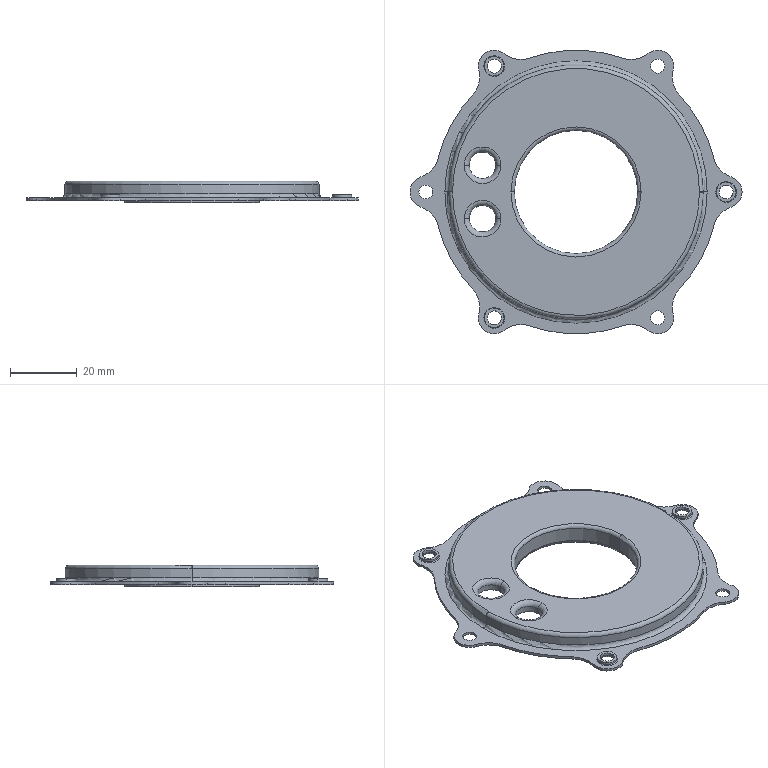Part | STEP file | JAIREIPAN_146_1_1 | 1 solid | 119 faces | box 99.5 x 85 x 6.5 mm | volume 5367 mm3 | cylinder 68 | torus 36 | plane 15 | commonest cylinder face diameters 4.2 x12 16 x12 3 x8 5.8 x6 9.5 x6 85 x6